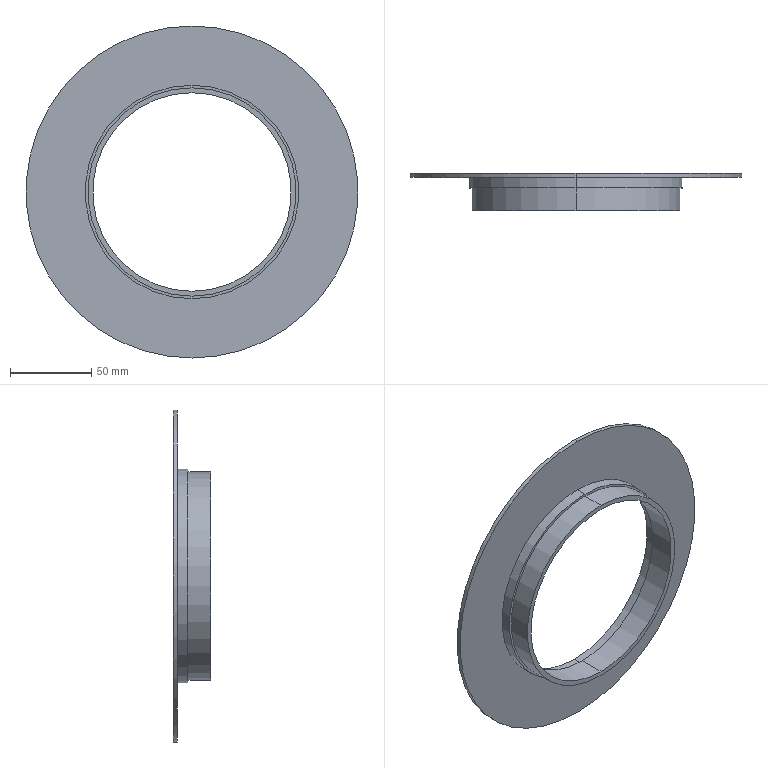Part | SolidWorks | features Revolution 1 | 1 solid | 15 faces | box 204 x 23.032 x 204 mm | volume 75722 mm3 | cylinder 10 | plane 5 | commonest cylinder face diameters 121.991 x2 126.387 x2 127.991 x2 131.166 x2 204 x2
STEP:
#1=CARTESIAN_POINT('',(0.,153.779,-63.194));
#2=VERTEX_POINT('',#1);
#3=CARTESIAN_POINT('',(0.,153.779,63.194));
#4=VERTEX_POINT('',#3);
#5=CARTESIAN_POINT('',(0.,153.779,0.));
#6=DIRECTION('',(0.,1.,0.));
#7=DIRECTION('',(0.,0.,1.));
#8=AXIS2_PLACEMENT_3D('',#5,#6,#7);
#9=CIRCLE('',#8,63.194);
#10=EDGE_CURVE('',#2,#4,#9,.T.);
#11=ORIENTED_EDGE('',*,*,#10,.F.);
#12=CARTESIAN_POINT('',(0.,160.532,-63.194));
#13=VERTEX_POINT('',#12);
#14=CARTESIAN_POINT('',(0.,0.,-63.194));
#15=DIRECTION('',(0.,1.,0.));
#16=VECTOR('',#15,1000.);
#17=LINE('',#14,#16);
#18=EDGE_CURVE('',#2,#13,#17,.T.);
#19=ORIENTED_EDGE('',*,*,#18,.T.);
#20=CARTESIAN_POINT('',(0.,160.532,63.194));
#21=VERTEX_POINT('',#20);
#22=CARTESIAN_POINT('',(0.,160.532,0.));
#23=DIRECTION('',(0.,1.,0.));
#24=DIRECTION('',(0.,0.,1.));
#25=AXIS2_PLACEMENT_3D('',#22,#23,#24);
#26=CIRCLE('',#25,63.194);
#27=EDGE_CURVE('',#13,#21,#26,.T.);
#28=ORIENTED_EDGE('',*,*,#27,.T.);
#29=CARTESIAN_POINT('',(0.,0.,63.194));
#30=DIRECTION('',(0.,1.,0.));
#31=VECTOR('',#30,1000.);
#32=LINE('',#29,#31);
#33=EDGE_CURVE('',#4,#21,#32,.T.);
#34=ORIENTED_EDGE('',*,*,#33,.F.);
#35=EDGE_LOOP('',(#11,#19,#28,#34));
#36=FACE_OUTER_BOUND('',#35,.T.);
#37=CARTESIAN_POINT('',(0.,0.,0.));
#38=DIRECTION('',(0.,1.,0.));
#39=DIRECTION('',(0.,0.,1.));
#40=AXIS2_PLACEMENT_3D('',#37,#38,#39);
#41=CYLINDRICAL_SURFACE('',#40,63.194);
#42=ADVANCED_FACE('',(#36),#41,.F.);
#43=CARTESIAN_POINT('',(0.,137.5,-60.996));
#44=VERTEX_POINT('',#43);
#45=CARTESIAN_POINT('',(0.,137.5,60.996));
#46=VERTEX_POINT('',#45);
#47=CARTESIAN_POINT('',(0.,137.5,0.));
#48=DIRECTION('',(0.,1.,0.));
#49=DIRECTION('',(0.,0.,1.));
#50=AXIS2_PLACEMENT_3D('',#47,#48,#49);
#51=CIRCLE('',#50,60.996);
#52=EDGE_CURVE('',#44,#46,#51,.T.);
#53=ORIENTED_EDGE('',*,*,#52,.F.);
#54=CARTESIAN_POINT('',(0.,153.779,-60.996));
#55=VERTEX_POINT('',#54);
#56=CARTESIAN_POINT('',(0.,0.,-60.996));
#57=DIRECTION('',(0.,1.,0.));
#58=VECTOR('',#57,1000.);
#59=LINE('',#56,#58);
#60=EDGE_CURVE('',#44,#55,#59,.T.);
#61=ORIENTED_EDGE('',*,*,#60,.T.);
#62=CARTESIAN_POINT('',(0.,153.779,60.996));
#63=VERTEX_POINT('',#62);
#64=CARTESIAN_POINT('',(0.,153.779,0.));
#65=DIRECTION('',(0.,1.,0.));
#66=DIRECTION('',(0.,0.,1.));
#67=AXIS2_PLACEMENT_3D('',#64,#65,#66);
#68=CIRCLE('',#67,60.996);
#69=EDGE_CURVE('',#55,#63,#68,.T.);
#70=ORIENTED_EDGE('',*,*,#69,.T.);
#71=CARTESIAN_POINT('',(0.,0.,60.996));
#72=DIRECTION('',(0.,1.,0.));
#73=VECTOR('',#72,1000.);
#74=LINE('',#71,#73);
#75=EDGE_CURVE('',#46,#63,#74,.T.);
#76=ORIENTED_EDGE('',*,*,#75,.F.);
#77=EDGE_LOOP('',(#53,#61,#70,#76));
#78=FACE_OUTER_BOUND('',#77,.T.);
#79=CARTESIAN_POINT('',(0.,0.,0.));
#80=DIRECTION('',(0.,1.,0.));
#81=DIRECTION('',(0.,0.,1.));
#82=AXIS2_PLACEMENT_3D('',#79,#80,#81);
#83=CYLINDRICAL_SURFACE('',#82,60.996);
#84=ADVANCED_FACE('',(#78),#83,.F.);
#85=CARTESIAN_POINT('',(0.,137.5,63.996));
#86=VERTEX_POINT('',#85);
#87=CARTESIAN_POINT('',(0.,137.5,-63.996));
#88=VERTEX_POINT('',#87);
#89=CARTESIAN_POINT('',(0.,137.5,0.));
#90=DIRECTION('',(0.,1.,0.));
#91=DIRECTION('',(0.,0.,1.));
#92=AXIS2_PLACEMENT_3D('',#89,#90,#91);
#93=CIRCLE('',#92,63.996);
#94=EDGE_CURVE('',#86,#88,#93,.T.);
#95=ORIENTED_EDGE('',*,*,#94,.T.);
#96=CARTESIAN_POINT('',(0.,151.5,-63.996));
#97=VERTEX_POINT('',#96);
#98=CARTESIAN_POINT('',(0.,0.,-63.996));
#99=DIRECTION('',(0.,1.,0.));
#100=VECTOR('',#99,1000.);
#101=LINE('',#98,#100);
#102=EDGE_CURVE('',#88,#97,#101,.T.);
#103=ORIENTED_EDGE('',*,*,#102,.T.);
#104=CARTESIAN_POINT('',(0.,151.5,63.996));
#105=VERTEX_POINT('',#104);
#106=CARTESIAN_POINT('',(0.,151.5,0.));
#107=DIRECTION('',(0.,1.,0.));
#108=DIRECTION('',(0.,0.,1.));
#109=AXIS2_PLACEMENT_3D('',#106,#107,#108);
#110=CIRCLE('',#109,63.996);
#111=EDGE_CURVE('',#105,#97,#110,.T.);
#112=ORIENTED_EDGE('',*,*,#111,.F.);
#113=CARTESIAN_POINT('',(0.,0.,63.996));
#114=DIRECTION('',(0.,1.,0.));
#115=VECTOR('',#114,1000.);
#116=LINE('',#113,#115);
#117=EDGE_CURVE('',#86,#105,#116,.T.);
#118=ORIENTED_EDGE('',*,*,#117,.F.);
#119=EDGE_LOOP('',(#95,#103,#112,#118));
#120=FACE_OUTER_BOUND('',#119,.T.);
#121=CARTESIAN_POINT('',(0.,0.,0.));
#122=DIRECTION('',(0.,1.,0.));
#123=DIRECTION('',(0.,0.,1.));
#124=AXIS2_PLACEMENT_3D('',#121,#122,#123);
#125=CYLINDRICAL_SURFACE('',#124,63.996);
#126=ADVANCED_FACE('',(#120),#125,.T.);
#127=CARTESIAN_POINT('',(0.,151.5,65.583));
#128=VERTEX_POINT('',#127);
#129=CARTESIAN_POINT('',(0.,151.5,-65.583));
#130=VERTEX_POINT('',#129);
#131=CARTESIAN_POINT('',(0.,151.5,0.));
#132=DIRECTION('',(0.,1.,0.));
#133=DIRECTION('',(0.,0.,1.));
#134=AXIS2_PLACEMENT_3D('',#131,#132,#133);
#135=CIRCLE('',#134,65.583);
#136=EDGE_CURVE('',#128,#130,#135,.T.);
#137=ORIENTED_EDGE('',*,*,#136,.T.);
#138=CARTESIAN_POINT('',(0.,158.,-65.583));
#139=VERTEX_POINT('',#138);
#140=CARTESIAN_POINT('',(0.,0.,-65.583));
#141=DIRECTION('',(0.,1.,0.));
#142=VECTOR('',#141,1000.);
#143=LINE('',#140,#142);
#144=EDGE_CURVE('',#130,#139,#143,.T.);
#145=ORIENTED_EDGE('',*,*,#144,.T.);
#146=CARTESIAN_POINT('',(0.,158.,65.583));
#147=VERTEX_POINT('',#146);
#148=CARTESIAN_POINT('',(0.,158.,0.));
#149=DIRECTION('',(0.,1.,0.));
#150=DIRECTION('',(0.,0.,1.));
#151=AXIS2_PLACEMENT_3D('',#148,#149,#150);
#152=CIRCLE('',#151,65.583);
#153=EDGE_CURVE('',#147,#139,#152,.T.);
#154=ORIENTED_EDGE('',*,*,#153,.F.);
#155=CARTESIAN_POINT('',(0.,0.,65.583));
#156=DIRECTION('',(0.,1.,0.));
#157=VECTOR('',#156,1000.);
#158=LINE('',#155,#157);
#159=EDGE_CURVE('',#128,#147,#158,.T.);
#160=ORIENTED_EDGE('',*,*,#159,.F.);
#161=EDGE_LOOP('',(#137,#145,#154,#160));
#162=FACE_OUTER_BOUND('',#161,.T.);
#163=CARTESIAN_POINT('',(0.,0.,0.));
#164=DIRECTION('',(0.,1.,0.));
#165=DIRECTION('',(0.,0.,1.));
#166=AXIS2_PLACEMENT_3D('',#163,#164,#165);
#167=CYLINDRICAL_SURFACE('',#166,65.583);
#168=ADVANCED_FACE('',(#162),#167,.T.);
#169=CARTESIAN_POINT('',(0.,158.,102.));
#170=VERTEX_POINT('',#169);
#171=CARTESIAN_POINT('',(0.,158.,-102.));
#172=VERTEX_POINT('',#171);
#173=CARTESIAN_POINT('',(0.,158.,0.));
#174=DIRECTION('',(0.,1.,0.));
#175=DIRECTION('',(0.,0.,1.));
#176=AXIS2_PLACEMENT_3D('',#173,#174,#175);
#177=CIRCLE('',#176,102.);
#178=EDGE_CURVE('',#170,#172,#177,.T.);
#179=ORIENTED_EDGE('',*,*,#178,.T.);
#180=CARTESIAN_POINT('',(0.,160.532,-102.));
#181=VERTEX_POINT('',#180);
#182=CARTESIAN_POINT('',(0.,0.,-102.));
#183=DIRECTION('',(0.,1.,0.));
#184=VECTOR('',#183,1000.);
#185=LINE('',#182,#184);
#186=EDGE_CURVE('',#172,#181,#185,.T.);
#187=ORIENTED_EDGE('',*,*,#186,.T.);
#188=CARTESIAN_POINT('',(0.,160.532,102.));
#189=VERTEX_POINT('',#188);
#190=CARTESIAN_POINT('',(0.,160.532,0.));
#191=DIRECTION('',(0.,1.,0.));
#192=DIRECTION('',(0.,0.,1.));
#193=AXIS2_PLACEMENT_3D('',#190,#191,#192);
#194=CIRCLE('',#193,102.);
#195=EDGE_CURVE('',#189,#181,#194,.T.);
#196=ORIENTED_EDGE('',*,*,#195,.F.);
#197=CARTESIAN_POINT('',(0.,0.,102.));
#198=DIRECTION('',(0.,1.,0.));
#199=VECTOR('',#198,1000.);
#200=LINE('',#197,#199);
#201=EDGE_CURVE('',#170,#189,#200,.T.);
#202=ORIENTED_EDGE('',*,*,#201,.F.);
#203=EDGE_LOOP('',(#179,#187,#196,#202));
#204=FACE_OUTER_BOUND('',#203,.T.);
#205=CARTESIAN_POINT('',(0.,0.,0.));
#206=DIRECTION('',(0.,1.,0.));
#207=DIRECTION('',(0.,0.,1.));
#208=AXIS2_PLACEMENT_3D('',#205,#206,#207);
#209=CYLINDRICAL_SURFACE('',#208,102.);
#210=ADVANCED_FACE('',(#204),#209,.T.);
#211=ORIENTED_EDGE('',*,*,#186,.F.);
#212=CARTESIAN_POINT('',(0.,158.,0.));
#213=DIRECTION('',(0.,1.,0.));
#214=DIRECTION('',(0.,0.,1.));
#215=AXIS2_PLACEMENT_3D('',#212,#213,#214);
#216=CIRCLE('',#215,102.);
#217=EDGE_CURVE('',#172,#170,#216,.T.);
#218=ORIENTED_EDGE('',*,*,#217,.T.);
#219=ORIENTED_EDGE('',*,*,#201,.T.);
#220=CARTESIAN_POINT('',(0.,160.532,0.));
#221=DIRECTION('',(0.,1.,0.));
#222=DIRECTION('',(0.,0.,1.));
#223=AXIS2_PLACEMENT_3D('',#220,#221,#222);
#224=CIRCLE('',#223,102.);
#225=EDGE_CURVE('',#181,#189,#224,.T.);
#226=ORIENTED_EDGE('',*,*,#225,.F.);
#227=EDGE_LOOP('',(#211,#218,#219,#226));
#228=FACE_OUTER_BOUND('',#227,.T.);
#229=CARTESIAN_POINT('',(0.,0.,0.));
#230=DIRECTION('',(0.,1.,0.));
#231=DIRECTION('',(0.,0.,1.));
#232=AXIS2_PLACEMENT_3D('',#229,#230,#231);
#233=CYLINDRICAL_SURFACE('',#232,102.);
#234=ADVANCED_FACE('',(#228),#233,.T.);
#235=ORIENTED_EDGE('',*,*,#178,.F.);
#236=ORIENTED_EDGE('',*,*,#217,.F.);
#237=EDGE_LOOP('',(#235,#236));
#238=FACE_OUTER_BOUND('',#237,.T.);
#239=ORIENTED_EDGE('',*,*,#153,.T.);
#240=CARTESIAN_POINT('',(0.,158.,0.));
#241=DIRECTION('',(0.,1.,0.));
#242=DIRECTION('',(0.,0.,1.));
#243=AXIS2_PLACEMENT_3D('',#240,#241,#242);
#244=CIRCLE('',#243,65.583);
#245=EDGE_CURVE('',#139,#147,#244,.T.);
#246=ORIENTED_EDGE('',*,*,#245,.T.);
#247=EDGE_LOOP('',(#239,#246));
#248=FACE_BOUND('',#247,.T.);
#249=CARTESIAN_POINT('',(102.,158.,0.));
#250=DIRECTION('',(0.,1.,0.));
#251=DIRECTION('',(0.,0.,1.));
#252=AXIS2_PLACEMENT_3D('',#249,#250,#251);
#253=PLANE('',#252);
#254=ADVANCED_FACE('',(#238,#248),#253,.F.);
#255=ORIENTED_EDGE('',*,*,#144,.F.);
#256=CARTESIAN_POINT('',(0.,151.5,0.));
#257=DIRECTION('',(0.,1.,0.));
#258=DIRECTION('',(0.,0.,1.));
#259=AXIS2_PLACEMENT_3D('',#256,#257,#258);
#260=CIRCLE('',#259,65.583);
#261=EDGE_CURVE('',#130,#128,#260,.T.);
#262=ORIENTED_EDGE('',*,*,#261,.T.);
#263=ORIENTED_EDGE('',*,*,#159,.T.);
#264=ORIENTED_EDGE('',*,*,#245,.F.);
#265=EDGE_LOOP('',(#255,#262,#263,#264));
#266=FACE_OUTER_BOUND('',#265,.T.);
#267=CARTESIAN_POINT('',(0.,0.,0.));
#268=DIRECTION('',(0.,1.,0.));
#269=DIRECTION('',(0.,0.,1.));
#270=AXIS2_PLACEMENT_3D('',#267,#268,#269);
#271=CYLINDRICAL_SURFACE('',#270,65.583);
#272=ADVANCED_FACE('',(#266),#271,.T.);
#273=ORIENTED_EDGE('',*,*,#136,.F.);
#274=ORIENTED_EDGE('',*,*,#261,.F.);
#275=EDGE_LOOP('',(#273,#274));
#276=FACE_OUTER_BOUND('',#275,.T.);
#277=ORIENTED_EDGE('',*,*,#111,.T.);
#278=CARTESIAN_POINT('',(0.,151.5,0.));
#279=DIRECTION('',(0.,1.,0.));
#280=DIRECTION('',(0.,0.,1.));
#281=AXIS2_PLACEMENT_3D('',#278,#279,#280);
#282=CIRCLE('',#281,63.996);
#283=EDGE_CURVE('',#97,#105,#282,.T.);
#284=ORIENTED_EDGE('',*,*,#283,.T.);
#285=EDGE_LOOP('',(#277,#284));
#286=FACE_BOUND('',#285,.T.);
#287=CARTESIAN_POINT('',(65.583,151.5,0.));
#288=DIRECTION('',(0.,1.,0.));
#289=DIRECTION('',(0.,0.,1.));
#290=AXIS2_PLACEMENT_3D('',#287,#288,#289);
#291=PLANE('',#290);
#292=ADVANCED_FACE('',(#276,#286),#291,.F.);
#293=ORIENTED_EDGE('',*,*,#102,.F.);
#294=CARTESIAN_POINT('',(0.,137.5,0.));
#295=DIRECTION('',(0.,1.,0.));
#296=DIRECTION('',(0.,0.,1.));
#297=AXIS2_PLACEMENT_3D('',#294,#295,#296);
#298=CIRCLE('',#297,63.996);
#299=EDGE_CURVE('',#88,#86,#298,.T.);
#300=ORIENTED_EDGE('',*,*,#299,.T.);
#301=ORIENTED_EDGE('',*,*,#117,.T.);
#302=ORIENTED_EDGE('',*,*,#283,.F.);
#303=EDGE_LOOP('',(#293,#300,#301,#302));
#304=FACE_OUTER_BOUND('',#303,.T.);
#305=CARTESIAN_POINT('',(0.,0.,0.));
#306=DIRECTION('',(0.,1.,0.));
#307=DIRECTION('',(0.,0.,1.));
#308=AXIS2_PLACEMENT_3D('',#305,#306,#307);
#309=CYLINDRICAL_SURFACE('',#308,63.996);
#310=ADVANCED_FACE('',(#304),#309,.T.);
#311=ORIENTED_EDGE('',*,*,#94,.F.);
#312=ORIENTED_EDGE('',*,*,#299,.F.);
#313=EDGE_LOOP('',(#311,#312));
#314=FACE_OUTER_BOUND('',#313,.T.);
#315=CARTESIAN_POINT('',(0.,137.5,0.));
#316=DIRECTION('',(0.,1.,0.));
#317=DIRECTION('',(0.,0.,1.));
#318=AXIS2_PLACEMENT_3D('',#315,#316,#317);
#319=CIRCLE('',#318,60.996);
#320=EDGE_CURVE('',#46,#44,#319,.T.);
#321=ORIENTED_EDGE('',*,*,#320,.T.);
#322=ORIENTED_EDGE('',*,*,#52,.T.);
#323=EDGE_LOOP('',(#321,#322));
#324=FACE_BOUND('',#323,.T.);
#325=CARTESIAN_POINT('',(63.996,137.5,0.));
#326=DIRECTION('',(0.,1.,0.));
#327=DIRECTION('',(0.,0.,1.));
#328=AXIS2_PLACEMENT_3D('',#325,#326,#327);
#329=PLANE('',#328);
#330=ADVANCED_FACE('',(#314,#324),#329,.F.);
#331=ORIENTED_EDGE('',*,*,#60,.F.);
#332=ORIENTED_EDGE('',*,*,#320,.F.);
#333=ORIENTED_EDGE('',*,*,#75,.T.);
#334=CARTESIAN_POINT('',(0.,153.779,0.));
#335=DIRECTION('',(0.,1.,0.));
#336=DIRECTION('',(0.,0.,1.));
#337=AXIS2_PLACEMENT_3D('',#334,#335,#336);
#338=CIRCLE('',#337,60.996);
#339=EDGE_CURVE('',#63,#55,#338,.T.);
#340=ORIENTED_EDGE('',*,*,#339,.T.);
#341=EDGE_LOOP('',(#331,#332,#333,#340));
#342=FACE_OUTER_BOUND('',#341,.T.);
#343=CARTESIAN_POINT('',(0.,0.,0.));
#344=DIRECTION('',(0.,1.,0.));
#345=DIRECTION('',(0.,0.,1.));
#346=AXIS2_PLACEMENT_3D('',#343,#344,#345);
#347=CYLINDRICAL_SURFACE('',#346,60.996);
#348=ADVANCED_FACE('',(#342),#347,.F.);
#349=ORIENTED_EDGE('',*,*,#339,.F.);
#350=ORIENTED_EDGE('',*,*,#69,.F.);
#351=EDGE_LOOP('',(#349,#350));
#352=FACE_BOUND('',#351,.T.);
#353=CARTESIAN_POINT('',(0.,153.779,0.));
#354=DIRECTION('',(0.,1.,0.));
#355=DIRECTION('',(0.,0.,1.));
#356=AXIS2_PLACEMENT_3D('',#353,#354,#355);
#357=CIRCLE('',#356,63.194);
#358=EDGE_CURVE('',#4,#2,#357,.T.);
#359=ORIENTED_EDGE('',*,*,#358,.T.);
#360=ORIENTED_EDGE('',*,*,#10,.T.);
#361=EDGE_LOOP('',(#359,#360));
#362=FACE_OUTER_BOUND('',#361,.T.);
#363=CARTESIAN_POINT('',(60.996,153.779,0.));
#364=DIRECTION('',(0.,-1.,0.));
#365=DIRECTION('',(0.,0.,-1.));
#366=AXIS2_PLACEMENT_3D('',#363,#364,#365);
#367=PLANE('',#366);
#368=ADVANCED_FACE('',(#352,#362),#367,.F.);
#369=ORIENTED_EDGE('',*,*,#18,.F.);
#370=ORIENTED_EDGE('',*,*,#358,.F.);
#371=ORIENTED_EDGE('',*,*,#33,.T.);
#372=CARTESIAN_POINT('',(0.,160.532,0.));
#373=DIRECTION('',(0.,1.,0.));
#374=DIRECTION('',(0.,0.,1.));
#375=AXIS2_PLACEMENT_3D('',#372,#373,#374);
#376=CIRCLE('',#375,63.194);
#377=EDGE_CURVE('',#21,#13,#376,.T.);
#378=ORIENTED_EDGE('',*,*,#377,.T.);
#379=EDGE_LOOP('',(#369,#370,#371,#378));
#380=FACE_OUTER_BOUND('',#379,.T.);
#381=CARTESIAN_POINT('',(0.,0.,0.));
#382=DIRECTION('',(0.,1.,0.));
#383=DIRECTION('',(0.,0.,1.));
#384=AXIS2_PLACEMENT_3D('',#381,#382,#383);
#385=CYLINDRICAL_SURFACE('',#384,63.194);
#386=ADVANCED_FACE('',(#380),#385,.F.);
#387=ORIENTED_EDGE('',*,*,#377,.F.);
#388=ORIENTED_EDGE('',*,*,#27,.F.);
#389=EDGE_LOOP('',(#387,#388));
#390=FACE_BOUND('',#389,.T.);
#391=ORIENTED_EDGE('',*,*,#195,.T.);
#392=ORIENTED_EDGE('',*,*,#225,.T.);
#393=EDGE_LOOP('',(#391,#392));
#394=FACE_OUTER_BOUND('',#393,.T.);
#395=CARTESIAN_POINT('',(63.194,160.532,0.));
#396=DIRECTION('',(0.,-1.,0.));
#397=DIRECTION('',(0.,0.,-1.));
#398=AXIS2_PLACEMENT_3D('',#395,#396,#397);
#399=PLANE('',#398);
#400=ADVANCED_FACE('',(#390,#394),#399,.F.);
#401=CLOSED_SHELL('',(#42,#84,#126,#168,#210,#234,#254,#272,#292,#310,#330,#348,#368,#386,#400));
#402=MANIFOLD_SOLID_BREP('',#401);
#403=CARTESIAN_POINT('',(0.,0.,0.));
#404=DIRECTION('',(0.,0.,1.));
#405=DIRECTION('',(1.,0.,0.));
#406=AXIS2_PLACEMENT_3D('',#403,#404,#405);
#407=(LENGTH_UNIT()NAMED_UNIT(*)SI_UNIT(.MILLI.,.METRE.));
#408=UNCERTAINTY_MEASURE_WITH_UNIT(LENGTH_MEASURE(0.00001),#407,'','');
#409=(NAMED_UNIT(*)PLANE_ANGLE_UNIT()SI_UNIT($,.RADIAN.));
#410=(NAMED_UNIT(*)SI_UNIT($,.STERADIAN.)SOLID_ANGLE_UNIT());
#411=(GEOMETRIC_REPRESENTATION_CONTEXT(3)GLOBAL_UNCERTAINTY_ASSIGNED_CONTEXT((#408))GLOBAL_UNIT_ASSIGNED_CONTEXT((#407,#409,#410))REPRESENTATION_CONTEXT('',''));
#412=ADVANCED_BREP_SHAPE_REPRESENTATION('',(#402,#406),#411);